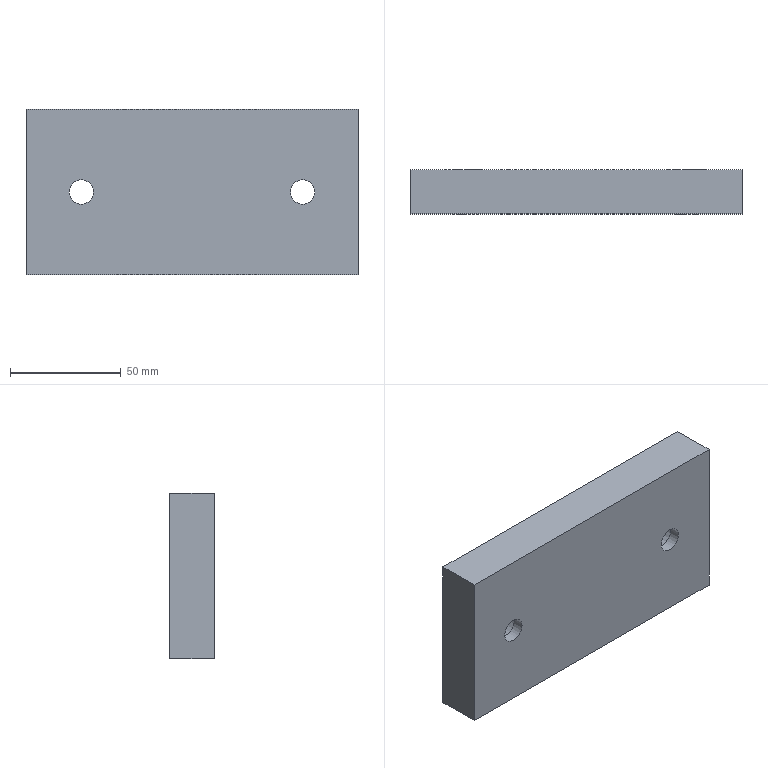Part | NX | features solid 2 | 1 solid | 12 faces | box 150 x 20 x 75 mm | volume 216834 mm3 | plane 8 | cylinder 4 | commonest cylinder face diameters 11 x2 17.5 x2
STEP:
#1=CARTESIAN_POINT('',(540.,1060.,-30.));
#2=VERTEX_POINT('',#1);
#3=CARTESIAN_POINT('',(540.,1060.,45.));
#4=VERTEX_POINT('',#3);
#5=CARTESIAN_POINT('',(540.,1060.,7.5));
#6=DIRECTION('',(0.,0.,1.));
#7=VECTOR('',#6,1000.);
#8=LINE('',#5,#7);
#9=EDGE_CURVE('',#2,#4,#8,.T.);
#10=ORIENTED_EDGE('',*,*,#9,.T.);
#11=CARTESIAN_POINT('',(540.,1040.,45.));
#12=VERTEX_POINT('',#11);
#13=CARTESIAN_POINT('',(540.,1050.,45.));
#14=DIRECTION('',(0.,-1.,0.));
#15=VECTOR('',#14,1000.);
#16=LINE('',#13,#15);
#17=EDGE_CURVE('',#4,#12,#16,.T.);
#18=ORIENTED_EDGE('',*,*,#17,.T.);
#19=CARTESIAN_POINT('',(540.,1040.,-30.));
#20=VERTEX_POINT('',#19);
#21=CARTESIAN_POINT('',(540.,1040.,7.5));
#22=DIRECTION('',(0.,0.,-1.));
#23=VECTOR('',#22,1000.);
#24=LINE('',#21,#23);
#25=EDGE_CURVE('',#12,#20,#24,.T.);
#26=ORIENTED_EDGE('',*,*,#25,.T.);
#27=CARTESIAN_POINT('',(540.,1050.,-30.));
#28=DIRECTION('',(0.,1.,0.));
#29=VECTOR('',#28,1000.);
#30=LINE('',#27,#29);
#31=EDGE_CURVE('',#20,#2,#30,.T.);
#32=ORIENTED_EDGE('',*,*,#31,.T.);
#33=EDGE_LOOP('',(#10,#18,#26,#32));
#34=FACE_BOUND('',#33,.T.);
#35=CARTESIAN_POINT('',(540.,1050.,7.5));
#36=DIRECTION('',(1.,0.,0.));
#37=DIRECTION('',(0.,0.,-1.));
#38=AXIS2_PLACEMENT_3D('',#35,#36,#37);
#39=PLANE('',#38);
#40=ADVANCED_FACE('',(#34),#39,.T.);
#41=CARTESIAN_POINT('',(423.75,1060.,7.5));
#42=VERTEX_POINT('',#41);
#43=CARTESIAN_POINT('',(415.,1060.,7.5));
#44=DIRECTION('',(0.,1.,0.));
#45=DIRECTION('',(1.,0.,0.));
#46=AXIS2_PLACEMENT_3D('',#43,#44,#45);
#47=CIRCLE('',#46,8.75);
#48=EDGE_CURVE('',#42,#42,#47,.T.);
#49=ORIENTED_EDGE('',*,*,#48,.F.);
#50=EDGE_LOOP('',(#49));
#51=FACE_BOUND('',#50,.T.);
#52=CARTESIAN_POINT('',(523.75,1060.,7.5));
#53=VERTEX_POINT('',#52);
#54=CARTESIAN_POINT('',(515.,1060.,7.5));
#55=DIRECTION('',(0.,1.,0.));
#56=DIRECTION('',(1.,0.,0.));
#57=AXIS2_PLACEMENT_3D('',#54,#55,#56);
#58=CIRCLE('',#57,8.75);
#59=EDGE_CURVE('',#53,#53,#58,.T.);
#60=ORIENTED_EDGE('',*,*,#59,.F.);
#61=EDGE_LOOP('',(#60));
#62=FACE_BOUND('',#61,.T.);
#63=CARTESIAN_POINT('',(390.,1060.,-30.));
#64=VERTEX_POINT('',#63);
#65=CARTESIAN_POINT('',(390.,1060.,-30.));
#66=DIRECTION('',(1.,0.,0.));
#67=VECTOR('',#66,1000.);
#68=LINE('',#65,#67);
#69=EDGE_CURVE('',#64,#2,#68,.T.);
#70=ORIENTED_EDGE('',*,*,#69,.F.);
#71=CARTESIAN_POINT('',(390.,1060.,45.));
#72=VERTEX_POINT('',#71);
#73=CARTESIAN_POINT('',(390.,1060.,7.5));
#74=DIRECTION('',(0.,0.,-1.));
#75=VECTOR('',#74,1000.);
#76=LINE('',#73,#75);
#77=EDGE_CURVE('',#72,#64,#76,.T.);
#78=ORIENTED_EDGE('',*,*,#77,.F.);
#79=CARTESIAN_POINT('',(390.,1060.,45.));
#80=DIRECTION('',(1.,0.,0.));
#81=VECTOR('',#80,1000.);
#82=LINE('',#79,#81);
#83=EDGE_CURVE('',#72,#4,#82,.T.);
#84=ORIENTED_EDGE('',*,*,#83,.T.);
#85=ORIENTED_EDGE('',*,*,#9,.F.);
#86=EDGE_LOOP('',(#70,#78,#84,#85));
#87=FACE_BOUND('',#86,.T.);
#88=CARTESIAN_POINT('',(390.,1060.,7.5));
#89=DIRECTION('',(0.,1.,0.));
#90=DIRECTION('',(-1.,0.,0.));
#91=AXIS2_PLACEMENT_3D('',#88,#89,#90);
#92=PLANE('',#91);
#93=ADVANCED_FACE('',(#51,#62,#87),#92,.T.);
#94=ORIENTED_EDGE('',*,*,#83,.F.);
#95=CARTESIAN_POINT('',(390.,1040.,45.));
#96=VERTEX_POINT('',#95);
#97=CARTESIAN_POINT('',(390.,1050.,45.));
#98=DIRECTION('',(0.,1.,0.));
#99=VECTOR('',#98,1000.);
#100=LINE('',#97,#99);
#101=EDGE_CURVE('',#96,#72,#100,.T.);
#102=ORIENTED_EDGE('',*,*,#101,.F.);
#103=CARTESIAN_POINT('',(390.,1040.,45.));
#104=DIRECTION('',(1.,0.,0.));
#105=VECTOR('',#104,1000.);
#106=LINE('',#103,#105);
#107=EDGE_CURVE('',#96,#12,#106,.T.);
#108=ORIENTED_EDGE('',*,*,#107,.T.);
#109=ORIENTED_EDGE('',*,*,#17,.F.);
#110=EDGE_LOOP('',(#94,#102,#108,#109));
#111=FACE_BOUND('',#110,.T.);
#112=CARTESIAN_POINT('',(390.,1050.,45.));
#113=DIRECTION('',(0.,0.,1.));
#114=DIRECTION('',(1.,0.,0.));
#115=AXIS2_PLACEMENT_3D('',#112,#113,#114);
#116=PLANE('',#115);
#117=ADVANCED_FACE('',(#111),#116,.T.);
#118=CARTESIAN_POINT('',(409.5,1040.,7.5));
#119=VERTEX_POINT('',#118);
#120=CARTESIAN_POINT('',(415.,1040.,7.5));
#121=DIRECTION('',(0.,-1.,0.));
#122=DIRECTION('',(-1.,0.,0.));
#123=AXIS2_PLACEMENT_3D('',#120,#121,#122);
#124=CIRCLE('',#123,5.5);
#125=EDGE_CURVE('',#119,#119,#124,.T.);
#126=ORIENTED_EDGE('',*,*,#125,.F.);
#127=EDGE_LOOP('',(#126));
#128=FACE_BOUND('',#127,.T.);
#129=CARTESIAN_POINT('',(509.5,1040.,7.5));
#130=VERTEX_POINT('',#129);
#131=CARTESIAN_POINT('',(515.,1040.,7.5));
#132=DIRECTION('',(0.,-1.,0.));
#133=DIRECTION('',(-1.,0.,0.));
#134=AXIS2_PLACEMENT_3D('',#131,#132,#133);
#135=CIRCLE('',#134,5.5);
#136=EDGE_CURVE('',#130,#130,#135,.T.);
#137=ORIENTED_EDGE('',*,*,#136,.F.);
#138=EDGE_LOOP('',(#137));
#139=FACE_BOUND('',#138,.T.);
#140=ORIENTED_EDGE('',*,*,#107,.F.);
#141=CARTESIAN_POINT('',(390.,1040.,-30.));
#142=VERTEX_POINT('',#141);
#143=CARTESIAN_POINT('',(390.,1040.,7.5));
#144=DIRECTION('',(0.,0.,1.));
#145=VECTOR('',#144,1000.);
#146=LINE('',#143,#145);
#147=EDGE_CURVE('',#142,#96,#146,.T.);
#148=ORIENTED_EDGE('',*,*,#147,.F.);
#149=CARTESIAN_POINT('',(390.,1040.,-30.));
#150=DIRECTION('',(1.,0.,0.));
#151=VECTOR('',#150,1000.);
#152=LINE('',#149,#151);
#153=EDGE_CURVE('',#142,#20,#152,.T.);
#154=ORIENTED_EDGE('',*,*,#153,.T.);
#155=ORIENTED_EDGE('',*,*,#25,.F.);
#156=EDGE_LOOP('',(#140,#148,#154,#155));
#157=FACE_BOUND('',#156,.T.);
#158=CARTESIAN_POINT('',(390.,1040.,7.5));
#159=DIRECTION('',(0.,-1.,0.));
#160=DIRECTION('',(1.,0.,0.));
#161=AXIS2_PLACEMENT_3D('',#158,#159,#160);
#162=PLANE('',#161);
#163=ADVANCED_FACE('',(#128,#139,#157),#162,.T.);
#164=CARTESIAN_POINT('',(390.,1050.,-30.));
#165=DIRECTION('',(0.,-1.,0.));
#166=VECTOR('',#165,1000.);
#167=LINE('',#164,#166);
#168=EDGE_CURVE('',#64,#142,#167,.T.);
#169=ORIENTED_EDGE('',*,*,#168,.T.);
#170=ORIENTED_EDGE('',*,*,#147,.T.);
#171=ORIENTED_EDGE('',*,*,#101,.T.);
#172=ORIENTED_EDGE('',*,*,#77,.T.);
#173=EDGE_LOOP('',(#169,#170,#171,#172));
#174=FACE_BOUND('',#173,.T.);
#175=CARTESIAN_POINT('',(390.,1050.,7.5));
#176=DIRECTION('',(-1.,0.,0.));
#177=DIRECTION('',(0.,0.,1.));
#178=AXIS2_PLACEMENT_3D('',#175,#176,#177);
#179=PLANE('',#178);
#180=ADVANCED_FACE('',(#174),#179,.T.);
#181=ORIENTED_EDGE('',*,*,#168,.F.);
#182=ORIENTED_EDGE('',*,*,#69,.T.);
#183=ORIENTED_EDGE('',*,*,#31,.F.);
#184=ORIENTED_EDGE('',*,*,#153,.F.);
#185=EDGE_LOOP('',(#181,#182,#183,#184));
#186=FACE_BOUND('',#185,.T.);
#187=CARTESIAN_POINT('',(390.,1050.,-30.));
#188=DIRECTION('',(0.,0.,-1.));
#189=DIRECTION('',(-1.,0.,0.));
#190=AXIS2_PLACEMENT_3D('',#187,#188,#189);
#191=PLANE('',#190);
#192=ADVANCED_FACE('',(#186),#191,.T.);
#193=CARTESIAN_POINT('',(520.5,1045.,7.5));
#194=VERTEX_POINT('',#193);
#195=CARTESIAN_POINT('',(515.,1045.,7.5));
#196=DIRECTION('',(0.,1.,0.));
#197=DIRECTION('',(1.,0.,0.));
#198=AXIS2_PLACEMENT_3D('',#195,#196,#197);
#199=CIRCLE('',#198,5.5);
#200=EDGE_CURVE('',#194,#194,#199,.F.);
#201=ORIENTED_EDGE('',*,*,#200,.F.);
#202=EDGE_LOOP('',(#201));
#203=FACE_BOUND('',#202,.T.);
#204=ORIENTED_EDGE('',*,*,#136,.T.);
#205=EDGE_LOOP('',(#204));
#206=FACE_BOUND('',#205,.T.);
#207=CARTESIAN_POINT('',(515.,1040.,7.5));
#208=DIRECTION('',(0.,1.,0.));
#209=DIRECTION('',(-1.,0.,0.));
#210=AXIS2_PLACEMENT_3D('',#207,#208,#209);
#211=CYLINDRICAL_SURFACE('',#210,5.5);
#212=ADVANCED_FACE('',(#203,#206),#211,.F.);
#213=CARTESIAN_POINT('',(506.25,1045.,7.5));
#214=VERTEX_POINT('',#213);
#215=CARTESIAN_POINT('',(515.,1045.,7.5));
#216=DIRECTION('',(0.,-1.,0.));
#217=DIRECTION('',(-1.,0.,0.));
#218=AXIS2_PLACEMENT_3D('',#215,#216,#217);
#219=CIRCLE('',#218,8.75);
#220=EDGE_CURVE('',#214,#214,#219,.T.);
#221=ORIENTED_EDGE('',*,*,#220,.F.);
#222=EDGE_LOOP('',(#221));
#223=FACE_BOUND('',#222,.T.);
#224=ORIENTED_EDGE('',*,*,#200,.T.);
#225=EDGE_LOOP('',(#224));
#226=FACE_BOUND('',#225,.T.);
#227=CARTESIAN_POINT('',(515.,1045.,7.5));
#228=DIRECTION('',(0.,-1.,0.));
#229=DIRECTION('',(1.,0.,0.));
#230=AXIS2_PLACEMENT_3D('',#227,#228,#229);
#231=PLANE('',#230);
#232=ADVANCED_FACE('',(#223,#226),#231,.F.);
#233=ORIENTED_EDGE('',*,*,#59,.T.);
#234=EDGE_LOOP('',(#233));
#235=FACE_BOUND('',#234,.T.);
#236=ORIENTED_EDGE('',*,*,#220,.T.);
#237=EDGE_LOOP('',(#236));
#238=FACE_BOUND('',#237,.T.);
#239=CARTESIAN_POINT('',(515.,1045.,7.5));
#240=DIRECTION('',(0.,1.,0.));
#241=DIRECTION('',(-1.,0.,0.));
#242=AXIS2_PLACEMENT_3D('',#239,#240,#241);
#243=CYLINDRICAL_SURFACE('',#242,8.75);
#244=ADVANCED_FACE('',(#235,#238),#243,.F.);
#245=CARTESIAN_POINT('',(420.5,1045.,7.5));
#246=VERTEX_POINT('',#245);
#247=CARTESIAN_POINT('',(415.,1045.,7.5));
#248=DIRECTION('',(0.,1.,0.));
#249=DIRECTION('',(1.,0.,0.));
#250=AXIS2_PLACEMENT_3D('',#247,#248,#249);
#251=CIRCLE('',#250,5.5);
#252=EDGE_CURVE('',#246,#246,#251,.F.);
#253=ORIENTED_EDGE('',*,*,#252,.F.);
#254=EDGE_LOOP('',(#253));
#255=FACE_BOUND('',#254,.T.);
#256=ORIENTED_EDGE('',*,*,#125,.T.);
#257=EDGE_LOOP('',(#256));
#258=FACE_BOUND('',#257,.T.);
#259=CARTESIAN_POINT('',(415.,1040.,7.5));
#260=DIRECTION('',(0.,1.,0.));
#261=DIRECTION('',(-1.,0.,0.));
#262=AXIS2_PLACEMENT_3D('',#259,#260,#261);
#263=CYLINDRICAL_SURFACE('',#262,5.5);
#264=ADVANCED_FACE('',(#255,#258),#263,.F.);
#265=CARTESIAN_POINT('',(406.25,1045.,7.5));
#266=VERTEX_POINT('',#265);
#267=CARTESIAN_POINT('',(415.,1045.,7.5));
#268=DIRECTION('',(0.,-1.,0.));
#269=DIRECTION('',(-1.,0.,0.));
#270=AXIS2_PLACEMENT_3D('',#267,#268,#269);
#271=CIRCLE('',#270,8.75);
#272=EDGE_CURVE('',#266,#266,#271,.T.);
#273=ORIENTED_EDGE('',*,*,#272,.F.);
#274=EDGE_LOOP('',(#273));
#275=FACE_BOUND('',#274,.T.);
#276=ORIENTED_EDGE('',*,*,#252,.T.);
#277=EDGE_LOOP('',(#276));
#278=FACE_BOUND('',#277,.T.);
#279=CARTESIAN_POINT('',(415.,1045.,7.5));
#280=DIRECTION('',(0.,-1.,0.));
#281=DIRECTION('',(1.,0.,0.));
#282=AXIS2_PLACEMENT_3D('',#279,#280,#281);
#283=PLANE('',#282);
#284=ADVANCED_FACE('',(#275,#278),#283,.F.);
#285=ORIENTED_EDGE('',*,*,#48,.T.);
#286=EDGE_LOOP('',(#285));
#287=FACE_BOUND('',#286,.T.);
#288=ORIENTED_EDGE('',*,*,#272,.T.);
#289=EDGE_LOOP('',(#288));
#290=FACE_BOUND('',#289,.T.);
#291=CARTESIAN_POINT('',(415.,1045.,7.5));
#292=DIRECTION('',(0.,1.,0.));
#293=DIRECTION('',(-1.,0.,0.));
#294=AXIS2_PLACEMENT_3D('',#291,#292,#293);
#295=CYLINDRICAL_SURFACE('',#294,8.75);
#296=ADVANCED_FACE('',(#287,#290),#295,.F.);
#297=CLOSED_SHELL('',(#40,#93,#117,#163,#180,#192,#212,#232,#244,#264,#284,#296));
#298=MANIFOLD_SOLID_BREP('',#297);
#299=(LENGTH_UNIT()NAMED_UNIT(*)SI_UNIT(.MILLI.,.METRE.));
#300=UNCERTAINTY_MEASURE_WITH_UNIT(LENGTH_MEASURE(0.00001),#299,'','');
#301=(NAMED_UNIT(*)PLANE_ANGLE_UNIT()SI_UNIT($,.RADIAN.));
#302=(NAMED_UNIT(*)SI_UNIT($,.STERADIAN.)SOLID_ANGLE_UNIT());
#303=(GEOMETRIC_REPRESENTATION_CONTEXT(3)GLOBAL_UNCERTAINTY_ASSIGNED_CONTEXT((#300))GLOBAL_UNIT_ASSIGNED_CONTEXT((#299,#301,#302))REPRESENTATION_CONTEXT('',''));
#304=ADVANCED_BREP_SHAPE_REPRESENTATION('',(#298),#303);